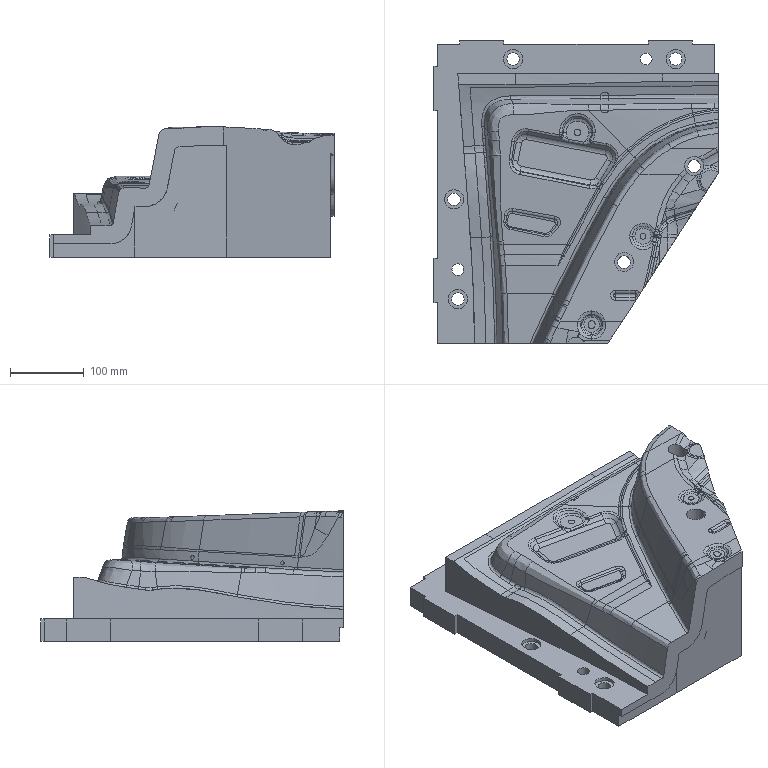Part | NX | features solid 2 | 1 solid | 359 faces | box 386.996 x 410.718 x 176.391 mm | volume 12393174 mm3 | spline 306 | plane 38 | cylinder 15 | commonest cylinder face diameters 26 x7 17 x6 16 x2